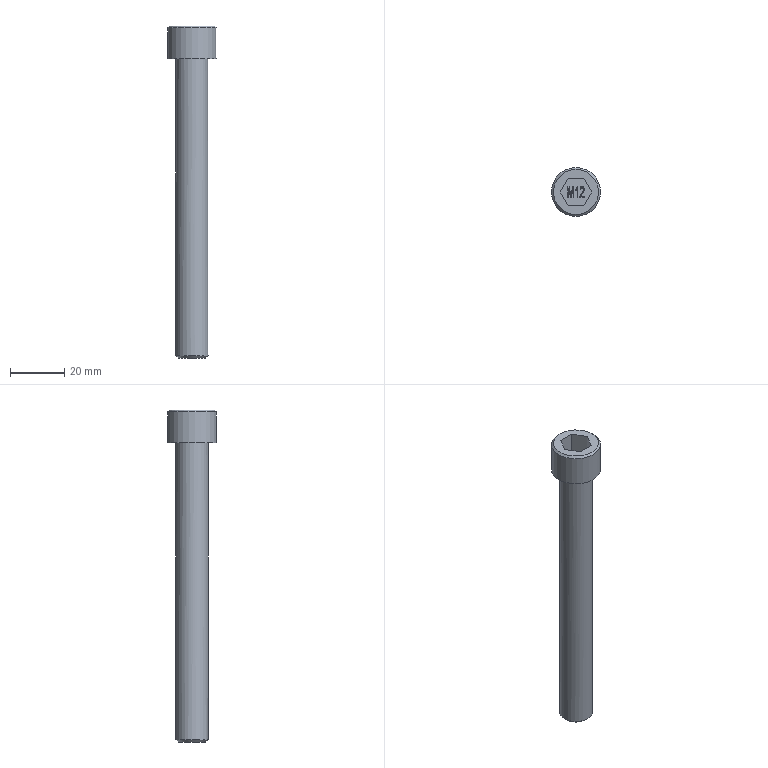Part | STEP file | EM11211000 | 1 solid | 43 faces | box 18 x 18 x 122 mm | volume 14775 mm3 | plane 33 | other 6 | cylinder 2 | cone 2 | commonest cylinder face diameters 12 x1 18 x1